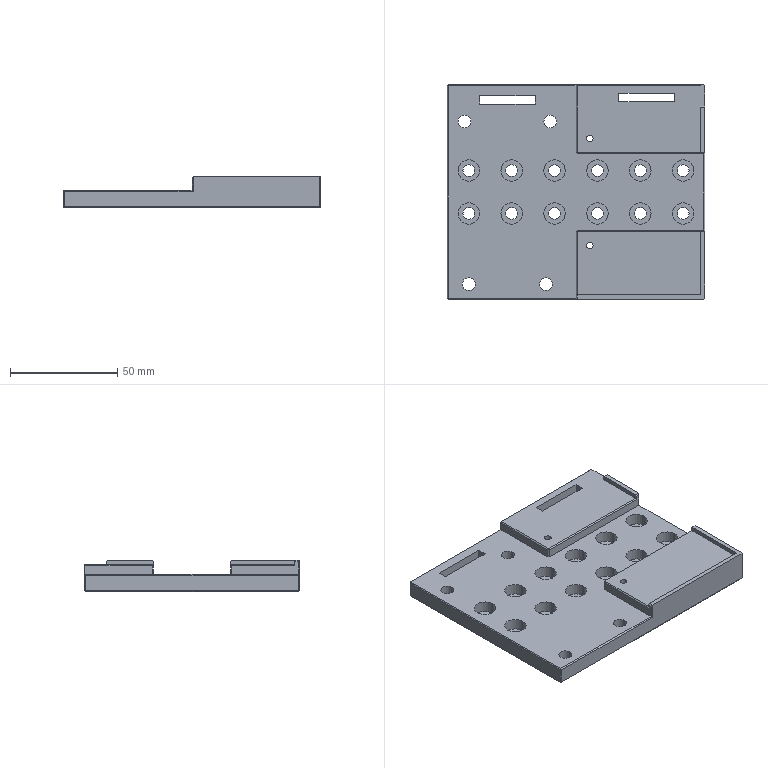Part | SolidWorks | features ICE 5, Chamfer 4, LPattern 3, HoleWzd 2, BaseBody 1, Cut 1, DelFace 1, Fillet 1 | 1 solid | 136 faces | box 120 x 100 x 14.5 mm | volume 104380 mm3 | plane 68 | cylinder 64 | cone 4 | commonest cylinder face diameters 5.5 x24 10 x24 6 x8 3 x4 3.3 x4